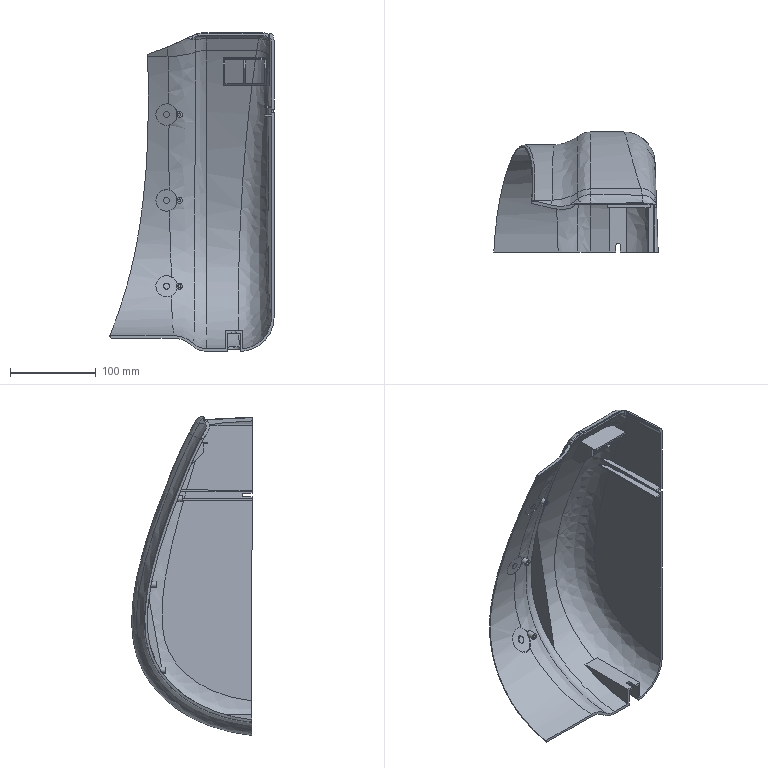Part | STEP file | MOTOR COVER R | 1 solid | 131 faces | box 191.608 x 140.54 x 371.606 mm | volume 329037 mm3 | spline 58 | plane 54 | cylinder 19 | commonest cylinder face diameters 7 x6 3.6 x3 25 x3 14 x2 16 x2 4 x1